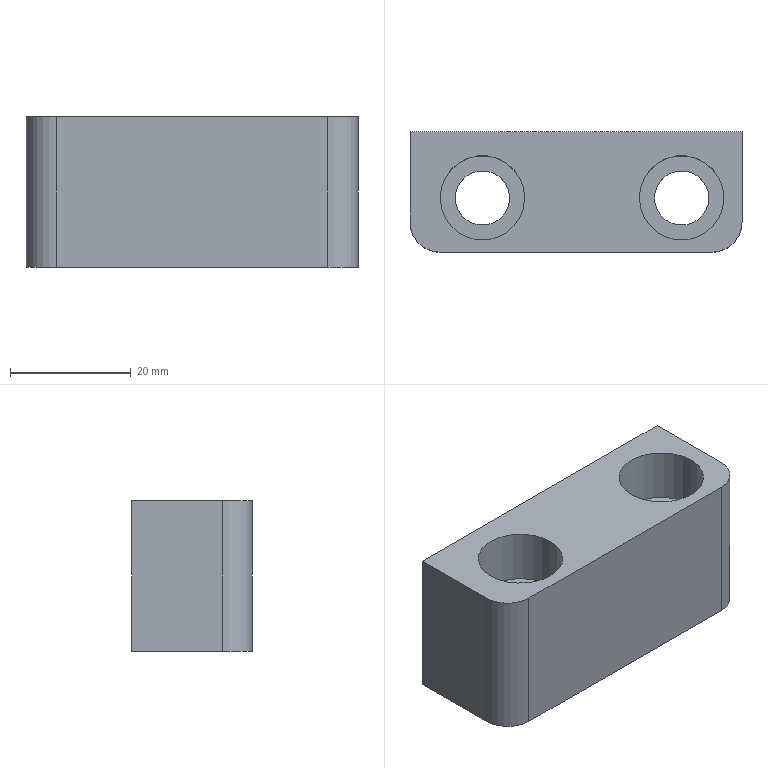Part | STEP file | solid 3 | 1 solid | 14 faces | box 55 x 20 x 25 mm | volume 22425 mm3 | plane 8 | cylinder 6 | commonest cylinder face diameters 9 x2 10 x2 14 x2